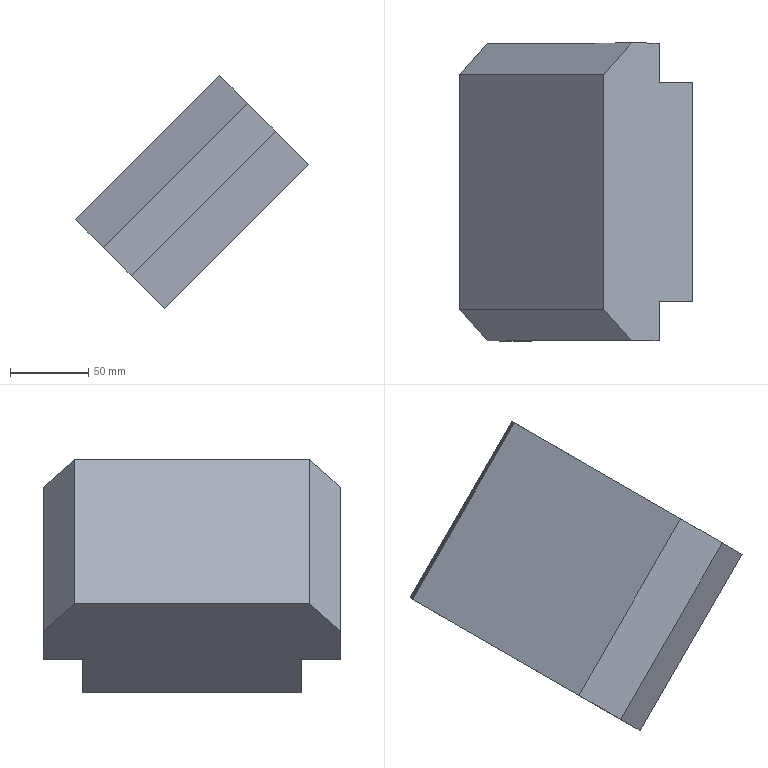Part | NX | features solid 2 | 1 solid | 12 faces | box 148.492 x 190 x 148.492 mm | volume 1716000 mm3 | plane 12
STEP:
#1=CARTESIAN_POINT('',(-990.395,255.,2.152));
#2=VERTEX_POINT('',#1);
#3=CARTESIAN_POINT('',(-990.395,105.,2.152));
#4=VERTEX_POINT('',#3);
#5=CARTESIAN_POINT('',(-990.395,255.,2.152));
#6=DIRECTION('',(0.,-1.,0.));
#7=VECTOR('',#6,1000.);
#8=LINE('',#5,#7);
#9=EDGE_CURVE('',#2,#4,#8,.T.);
#10=ORIENTED_EDGE('',*,*,#9,.F.);
#11=CARTESIAN_POINT('',(-1082.319,255.,-89.772));
#12=VERTEX_POINT('',#11);
#13=CARTESIAN_POINT('',(-1082.319,255.,-89.772));
#14=DIRECTION('',(0.7071,0.,0.7071));
#15=VECTOR('',#14,1000.);
#16=LINE('',#13,#15);
#17=EDGE_CURVE('',#12,#2,#16,.T.);
#18=ORIENTED_EDGE('',*,*,#17,.F.);
#19=CARTESIAN_POINT('',(-1082.319,105.,-89.772));
#20=VERTEX_POINT('',#19);
#21=CARTESIAN_POINT('',(-1082.319,255.,-89.772));
#22=DIRECTION('',(0.,-1.,0.));
#23=VECTOR('',#22,1000.);
#24=LINE('',#21,#23);
#25=EDGE_CURVE('',#12,#20,#24,.T.);
#26=ORIENTED_EDGE('',*,*,#25,.T.);
#27=CARTESIAN_POINT('',(-1082.319,105.,-89.772));
#28=DIRECTION('',(0.7071,0.,0.7071));
#29=VECTOR('',#28,1000.);
#30=LINE('',#27,#29);
#31=EDGE_CURVE('',#20,#4,#30,.T.);
#32=ORIENTED_EDGE('',*,*,#31,.T.);
#33=EDGE_LOOP('',(#10,#18,#26,#32));
#34=FACE_BOUND('',#33,.T.);
#35=CARTESIAN_POINT('',(-1082.319,255.,-89.772));
#36=DIRECTION('',(-0.7071,0.,0.7071));
#37=DIRECTION('',(-0.7071,0.,-0.7071));
#38=AXIS2_PLACEMENT_3D('',#35,#36,#37);
#39=PLANE('',#38);
#40=ADVANCED_FACE('',(#34),#39,.T.);
#41=CARTESIAN_POINT('',(-972.717,85.,-15.526));
#42=VERTEX_POINT('',#41);
#43=CARTESIAN_POINT('',(-990.395,105.,2.152));
#44=DIRECTION('',(0.5522,-0.6247,-0.5522));
#45=VECTOR('',#44,1000.);
#46=LINE('',#43,#45);
#47=EDGE_CURVE('',#4,#42,#46,.T.);
#48=ORIENTED_EDGE('',*,*,#47,.F.);
#49=ORIENTED_EDGE('',*,*,#31,.F.);
#50=CARTESIAN_POINT('',(-1064.641,85.,-107.45));
#51=VERTEX_POINT('',#50);
#52=CARTESIAN_POINT('',(-1082.319,105.,-89.772));
#53=DIRECTION('',(0.5522,-0.6247,-0.5522));
#54=VECTOR('',#53,1000.);
#55=LINE('',#52,#54);
#56=EDGE_CURVE('',#20,#51,#55,.T.);
#57=ORIENTED_EDGE('',*,*,#56,.T.);
#58=CARTESIAN_POINT('',(-1064.641,85.,-107.45));
#59=DIRECTION('',(0.7071,0.,0.7071));
#60=VECTOR('',#59,1000.);
#61=LINE('',#58,#60);
#62=EDGE_CURVE('',#51,#42,#61,.T.);
#63=ORIENTED_EDGE('',*,*,#62,.T.);
#64=EDGE_LOOP('',(#48,#49,#57,#63));
#65=FACE_BOUND('',#64,.T.);
#66=CARTESIAN_POINT('',(-1082.319,105.,-89.772));
#67=DIRECTION('',(-0.4417,-0.7809,0.4417));
#68=DIRECTION('',(0.07333,-0.5221,-0.8497));
#69=AXIS2_PLACEMENT_3D('',#66,#67,#68);
#70=PLANE('',#69);
#71=ADVANCED_FACE('',(#65),#70,.T.);
#72=CARTESIAN_POINT('',(-955.04,85.,-33.203));
#73=VERTEX_POINT('',#72);
#74=CARTESIAN_POINT('',(-972.717,85.,-15.526));
#75=DIRECTION('',(0.7071,0.,-0.7071));
#76=VECTOR('',#75,1000.);
#77=LINE('',#74,#76);
#78=EDGE_CURVE('',#42,#73,#77,.T.);
#79=ORIENTED_EDGE('',*,*,#78,.F.);
#80=ORIENTED_EDGE('',*,*,#62,.F.);
#81=CARTESIAN_POINT('',(-1046.964,85.,-125.127));
#82=VERTEX_POINT('',#81);
#83=CARTESIAN_POINT('',(-1064.641,85.,-107.45));
#84=DIRECTION('',(0.7071,0.,-0.7071));
#85=VECTOR('',#84,1000.);
#86=LINE('',#83,#85);
#87=EDGE_CURVE('',#51,#82,#86,.T.);
#88=ORIENTED_EDGE('',*,*,#87,.T.);
#89=CARTESIAN_POINT('',(-1046.964,85.,-125.127));
#90=DIRECTION('',(0.7071,0.,0.7071));
#91=VECTOR('',#90,1000.);
#92=LINE('',#89,#91);
#93=EDGE_CURVE('',#82,#73,#92,.T.);
#94=ORIENTED_EDGE('',*,*,#93,.T.);
#95=EDGE_LOOP('',(#79,#80,#88,#94));
#96=FACE_BOUND('',#95,.T.);
#97=CARTESIAN_POINT('',(-1064.641,85.,-107.45));
#98=DIRECTION('',(0.,-1.,0.));
#99=DIRECTION('',(0.9963,0.,0.08598));
#100=AXIS2_PLACEMENT_3D('',#97,#98,#99);
#101=PLANE('',#100);
#102=ADVANCED_FACE('',(#96),#101,.T.);
#103=CARTESIAN_POINT('',(-955.04,110.,-33.203));
#104=VERTEX_POINT('',#103);
#105=CARTESIAN_POINT('',(-955.04,85.,-33.203));
#106=DIRECTION('',(0.,1.,0.));
#107=VECTOR('',#106,1000.);
#108=LINE('',#105,#107);
#109=EDGE_CURVE('',#73,#104,#108,.T.);
#110=ORIENTED_EDGE('',*,*,#109,.F.);
#111=ORIENTED_EDGE('',*,*,#93,.F.);
#112=CARTESIAN_POINT('',(-1046.964,110.,-125.127));
#113=VERTEX_POINT('',#112);
#114=CARTESIAN_POINT('',(-1046.964,85.,-125.127));
#115=DIRECTION('',(0.,1.,0.));
#116=VECTOR('',#115,1000.);
#117=LINE('',#114,#116);
#118=EDGE_CURVE('',#82,#113,#117,.T.);
#119=ORIENTED_EDGE('',*,*,#118,.T.);
#120=CARTESIAN_POINT('',(-1046.964,110.,-125.127));
#121=DIRECTION('',(0.7071,0.,0.7071));
#122=VECTOR('',#121,1000.);
#123=LINE('',#120,#122);
#124=EDGE_CURVE('',#113,#104,#123,.T.);
#125=ORIENTED_EDGE('',*,*,#124,.T.);
#126=EDGE_LOOP('',(#110,#111,#119,#125));
#127=FACE_BOUND('',#126,.T.);
#128=CARTESIAN_POINT('',(-1046.964,85.,-125.127));
#129=DIRECTION('',(0.7071,0.,-0.7071));
#130=DIRECTION('',(0.7071,0.,0.7071));
#131=AXIS2_PLACEMENT_3D('',#128,#129,#130);
#132=PLANE('',#131);
#133=ADVANCED_FACE('',(#127),#132,.T.);
#134=CARTESIAN_POINT('',(-933.827,110.,-54.417));
#135=VERTEX_POINT('',#134);
#136=CARTESIAN_POINT('',(-955.04,110.,-33.203));
#137=DIRECTION('',(0.7071,0.,-0.7071));
#138=VECTOR('',#137,1000.);
#139=LINE('',#136,#138);
#140=EDGE_CURVE('',#104,#135,#139,.T.);
#141=ORIENTED_EDGE('',*,*,#140,.F.);
#142=ORIENTED_EDGE('',*,*,#124,.F.);
#143=CARTESIAN_POINT('',(-1025.75,110.,-146.34));
#144=VERTEX_POINT('',#143);
#145=CARTESIAN_POINT('',(-1046.964,110.,-125.127));
#146=DIRECTION('',(0.7071,0.,-0.7071));
#147=VECTOR('',#146,1000.);
#148=LINE('',#145,#147);
#149=EDGE_CURVE('',#113,#144,#148,.T.);
#150=ORIENTED_EDGE('',*,*,#149,.T.);
#151=CARTESIAN_POINT('',(-1025.75,110.,-146.34));
#152=DIRECTION('',(0.7071,0.,0.7071));
#153=VECTOR('',#152,1000.);
#154=LINE('',#151,#153);
#155=EDGE_CURVE('',#144,#135,#154,.T.);
#156=ORIENTED_EDGE('',*,*,#155,.T.);
#157=EDGE_LOOP('',(#141,#142,#150,#156));
#158=FACE_BOUND('',#157,.T.);
#159=CARTESIAN_POINT('',(-1046.964,110.,-125.127));
#160=DIRECTION('',(0.,-1.,0.));
#161=DIRECTION('',(0.08598,0.,-0.9963));
#162=AXIS2_PLACEMENT_3D('',#159,#160,#161);
#163=PLANE('',#162);
#164=ADVANCED_FACE('',(#158),#163,.T.);
#165=CARTESIAN_POINT('',(-933.827,250.,-54.417));
#166=VERTEX_POINT('',#165);
#167=CARTESIAN_POINT('',(-933.827,110.,-54.417));
#168=DIRECTION('',(0.,1.,0.));
#169=VECTOR('',#168,1000.);
#170=LINE('',#167,#169);
#171=EDGE_CURVE('',#135,#166,#170,.T.);
#172=ORIENTED_EDGE('',*,*,#171,.F.);
#173=ORIENTED_EDGE('',*,*,#155,.F.);
#174=CARTESIAN_POINT('',(-1025.75,250.,-146.34));
#175=VERTEX_POINT('',#174);
#176=CARTESIAN_POINT('',(-1025.75,110.,-146.34));
#177=DIRECTION('',(0.,1.,0.));
#178=VECTOR('',#177,1000.);
#179=LINE('',#176,#178);
#180=EDGE_CURVE('',#144,#175,#179,.T.);
#181=ORIENTED_EDGE('',*,*,#180,.T.);
#182=CARTESIAN_POINT('',(-1025.75,250.,-146.34));
#183=DIRECTION('',(0.7071,0.,0.7071));
#184=VECTOR('',#183,1000.);
#185=LINE('',#182,#184);
#186=EDGE_CURVE('',#175,#166,#185,.T.);
#187=ORIENTED_EDGE('',*,*,#186,.T.);
#188=EDGE_LOOP('',(#172,#173,#181,#187));
#189=FACE_BOUND('',#188,.T.);
#190=CARTESIAN_POINT('',(-1025.75,110.,-146.34));
#191=DIRECTION('',(0.7071,0.,-0.7071));
#192=DIRECTION('',(0.7071,0.,0.7071));
#193=AXIS2_PLACEMENT_3D('',#190,#191,#192);
#194=PLANE('',#193);
#195=ADVANCED_FACE('',(#189),#194,.T.);
#196=CARTESIAN_POINT('',(-955.04,250.,-33.203));
#197=VERTEX_POINT('',#196);
#198=CARTESIAN_POINT('',(-933.827,250.,-54.417));
#199=DIRECTION('',(-0.7071,0.,0.7071));
#200=VECTOR('',#199,1000.);
#201=LINE('',#198,#200);
#202=EDGE_CURVE('',#166,#197,#201,.T.);
#203=ORIENTED_EDGE('',*,*,#202,.F.);
#204=ORIENTED_EDGE('',*,*,#186,.F.);
#205=CARTESIAN_POINT('',(-1046.964,250.,-125.127));
#206=VERTEX_POINT('',#205);
#207=CARTESIAN_POINT('',(-1025.75,250.,-146.34));
#208=DIRECTION('',(-0.7071,0.,0.7071));
#209=VECTOR('',#208,1000.);
#210=LINE('',#207,#209);
#211=EDGE_CURVE('',#175,#206,#210,.T.);
#212=ORIENTED_EDGE('',*,*,#211,.T.);
#213=CARTESIAN_POINT('',(-1046.964,250.,-125.127));
#214=DIRECTION('',(0.7071,0.,0.7071));
#215=VECTOR('',#214,1000.);
#216=LINE('',#213,#215);
#217=EDGE_CURVE('',#206,#197,#216,.T.);
#218=ORIENTED_EDGE('',*,*,#217,.T.);
#219=EDGE_LOOP('',(#203,#204,#212,#218));
#220=FACE_BOUND('',#219,.T.);
#221=CARTESIAN_POINT('',(-1025.75,250.,-146.34));
#222=DIRECTION('',(0.,1.,0.));
#223=DIRECTION('',(-0.08598,0.,0.9963));
#224=AXIS2_PLACEMENT_3D('',#221,#222,#223);
#225=PLANE('',#224);
#226=ADVANCED_FACE('',(#220),#225,.T.);
#227=CARTESIAN_POINT('',(-955.04,275.,-33.203));
#228=VERTEX_POINT('',#227);
#229=CARTESIAN_POINT('',(-955.04,250.,-33.203));
#230=DIRECTION('',(0.,1.,0.));
#231=VECTOR('',#230,1000.);
#232=LINE('',#229,#231);
#233=EDGE_CURVE('',#197,#228,#232,.T.);
#234=ORIENTED_EDGE('',*,*,#233,.F.);
#235=ORIENTED_EDGE('',*,*,#217,.F.);
#236=CARTESIAN_POINT('',(-1046.964,275.,-125.127));
#237=VERTEX_POINT('',#236);
#238=CARTESIAN_POINT('',(-1046.964,250.,-125.127));
#239=DIRECTION('',(0.,1.,0.));
#240=VECTOR('',#239,1000.);
#241=LINE('',#238,#240);
#242=EDGE_CURVE('',#206,#237,#241,.T.);
#243=ORIENTED_EDGE('',*,*,#242,.T.);
#244=CARTESIAN_POINT('',(-1046.964,275.,-125.127));
#245=DIRECTION('',(0.7071,0.,0.7071));
#246=VECTOR('',#245,1000.);
#247=LINE('',#244,#246);
#248=EDGE_CURVE('',#237,#228,#247,.T.);
#249=ORIENTED_EDGE('',*,*,#248,.T.);
#250=EDGE_LOOP('',(#234,#235,#243,#249));
#251=FACE_BOUND('',#250,.T.);
#252=CARTESIAN_POINT('',(-1046.964,250.,-125.127));
#253=DIRECTION('',(0.7071,0.,-0.7071));
#254=DIRECTION('',(0.7071,0.,0.7071));
#255=AXIS2_PLACEMENT_3D('',#252,#253,#254);
#256=PLANE('',#255);
#257=ADVANCED_FACE('',(#251),#256,.T.);
#258=CARTESIAN_POINT('',(-972.717,275.,-15.526));
#259=VERTEX_POINT('',#258);
#260=CARTESIAN_POINT('',(-955.04,275.,-33.203));
#261=DIRECTION('',(-0.7071,0.,0.7071));
#262=VECTOR('',#261,1000.);
#263=LINE('',#260,#262);
#264=EDGE_CURVE('',#228,#259,#263,.T.);
#265=ORIENTED_EDGE('',*,*,#264,.F.);
#266=ORIENTED_EDGE('',*,*,#248,.F.);
#267=CARTESIAN_POINT('',(-1064.641,275.,-107.45));
#268=VERTEX_POINT('',#267);
#269=CARTESIAN_POINT('',(-1046.964,275.,-125.127));
#270=DIRECTION('',(-0.7071,0.,0.7071));
#271=VECTOR('',#270,1000.);
#272=LINE('',#269,#271);
#273=EDGE_CURVE('',#237,#268,#272,.T.);
#274=ORIENTED_EDGE('',*,*,#273,.T.);
#275=CARTESIAN_POINT('',(-1064.641,275.,-107.45));
#276=DIRECTION('',(0.7071,0.,0.7071));
#277=VECTOR('',#276,1000.);
#278=LINE('',#275,#277);
#279=EDGE_CURVE('',#268,#259,#278,.T.);
#280=ORIENTED_EDGE('',*,*,#279,.T.);
#281=EDGE_LOOP('',(#265,#266,#274,#280));
#282=FACE_BOUND('',#281,.T.);
#283=CARTESIAN_POINT('',(-1046.964,275.,-125.127));
#284=DIRECTION('',(0.,1.,0.));
#285=DIRECTION('',(-0.9963,0.,-0.08598));
#286=AXIS2_PLACEMENT_3D('',#283,#284,#285);
#287=PLANE('',#286);
#288=ADVANCED_FACE('',(#282),#287,.T.);
#289=CARTESIAN_POINT('',(-972.717,275.,-15.526));
#290=DIRECTION('',(-0.5522,-0.6247,0.5522));
#291=VECTOR('',#290,1000.);
#292=LINE('',#289,#291);
#293=EDGE_CURVE('',#259,#2,#292,.T.);
#294=ORIENTED_EDGE('',*,*,#293,.F.);
#295=ORIENTED_EDGE('',*,*,#279,.F.);
#296=CARTESIAN_POINT('',(-1064.641,275.,-107.45));
#297=DIRECTION('',(-0.5522,-0.6247,0.5522));
#298=VECTOR('',#297,1000.);
#299=LINE('',#296,#298);
#300=EDGE_CURVE('',#268,#12,#299,.T.);
#301=ORIENTED_EDGE('',*,*,#300,.T.);
#302=ORIENTED_EDGE('',*,*,#17,.T.);
#303=EDGE_LOOP('',(#294,#295,#301,#302));
#304=FACE_BOUND('',#303,.T.);
#305=CARTESIAN_POINT('',(-1064.641,275.,-107.45));
#306=DIRECTION('',(-0.4417,0.7809,0.4417));
#307=DIRECTION('',(-0.07333,-0.5221,0.8497));
#308=AXIS2_PLACEMENT_3D('',#305,#306,#307);
#309=PLANE('',#308);
#310=ADVANCED_FACE('',(#304),#309,.T.);
#311=ORIENTED_EDGE('',*,*,#25,.F.);
#312=ORIENTED_EDGE('',*,*,#300,.F.);
#313=ORIENTED_EDGE('',*,*,#273,.F.);
#314=ORIENTED_EDGE('',*,*,#242,.F.);
#315=ORIENTED_EDGE('',*,*,#211,.F.);
#316=ORIENTED_EDGE('',*,*,#180,.F.);
#317=ORIENTED_EDGE('',*,*,#149,.F.);
#318=ORIENTED_EDGE('',*,*,#118,.F.);
#319=ORIENTED_EDGE('',*,*,#87,.F.);
#320=ORIENTED_EDGE('',*,*,#56,.F.);
#321=EDGE_LOOP('',(#311,#312,#313,#314,#315,#316,#317,#318,#319,#320));
#322=FACE_BOUND('',#321,.T.);
#323=CARTESIAN_POINT('',(-1082.319,85.,-89.772));
#324=DIRECTION('',(0.7071,0.,0.7071));
#325=DIRECTION('',(-0.7071,0.,0.7071));
#326=AXIS2_PLACEMENT_3D('',#323,#324,#325);
#327=PLANE('',#326);
#328=ADVANCED_FACE('',(#322),#327,.F.);
#329=ORIENTED_EDGE('',*,*,#9,.T.);
#330=ORIENTED_EDGE('',*,*,#47,.T.);
#331=ORIENTED_EDGE('',*,*,#78,.T.);
#332=ORIENTED_EDGE('',*,*,#109,.T.);
#333=ORIENTED_EDGE('',*,*,#140,.T.);
#334=ORIENTED_EDGE('',*,*,#171,.T.);
#335=ORIENTED_EDGE('',*,*,#202,.T.);
#336=ORIENTED_EDGE('',*,*,#233,.T.);
#337=ORIENTED_EDGE('',*,*,#264,.T.);
#338=ORIENTED_EDGE('',*,*,#293,.T.);
#339=EDGE_LOOP('',(#329,#330,#331,#332,#333,#334,#335,#336,#337,#338));
#340=FACE_BOUND('',#339,.T.);
#341=CARTESIAN_POINT('',(-990.395,85.,2.152));
#342=DIRECTION('',(0.7071,0.,0.7071));
#343=DIRECTION('',(-0.7071,0.,0.7071));
#344=AXIS2_PLACEMENT_3D('',#341,#342,#343);
#345=PLANE('',#344);
#346=ADVANCED_FACE('',(#340),#345,.T.);
#347=CLOSED_SHELL('',(#40,#71,#102,#133,#164,#195,#226,#257,#288,#310,#328,#346));
#348=MANIFOLD_SOLID_BREP('',#347);
#349=(LENGTH_UNIT()NAMED_UNIT(*)SI_UNIT(.MILLI.,.METRE.));
#350=UNCERTAINTY_MEASURE_WITH_UNIT(LENGTH_MEASURE(0.00001),#349,'','');
#351=(NAMED_UNIT(*)PLANE_ANGLE_UNIT()SI_UNIT($,.RADIAN.));
#352=(NAMED_UNIT(*)SI_UNIT($,.STERADIAN.)SOLID_ANGLE_UNIT());
#353=(GEOMETRIC_REPRESENTATION_CONTEXT(3)GLOBAL_UNCERTAINTY_ASSIGNED_CONTEXT((#350))GLOBAL_UNIT_ASSIGNED_CONTEXT((#349,#351,#352))REPRESENTATION_CONTEXT('',''));
#354=ADVANCED_BREP_SHAPE_REPRESENTATION('',(#348),#353);